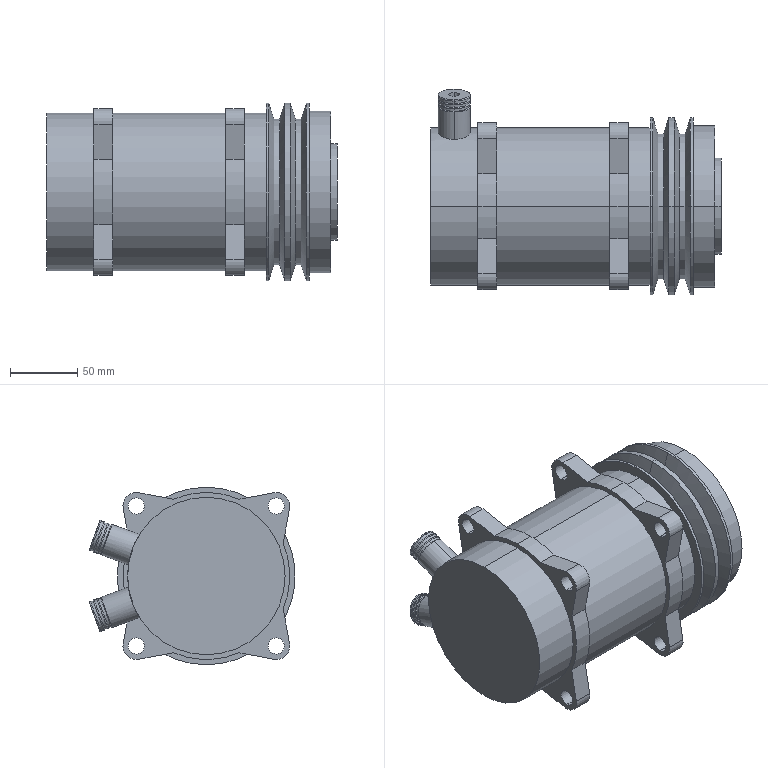Part | SolidWorks | features MirrorPattern 3, ICE 2, Revolution 2, Extrusion 1, LPattern 1 | 1 solid | 134 faces | box 216 x 153.032 x 132 mm | volume 2427701 mm3 | cylinder 82 | plane 28 | torus 16 | cone 8 | commonest cylinder face diameters 12 x16 20 x12 23 x12 124 x10 117 x8 132 x6